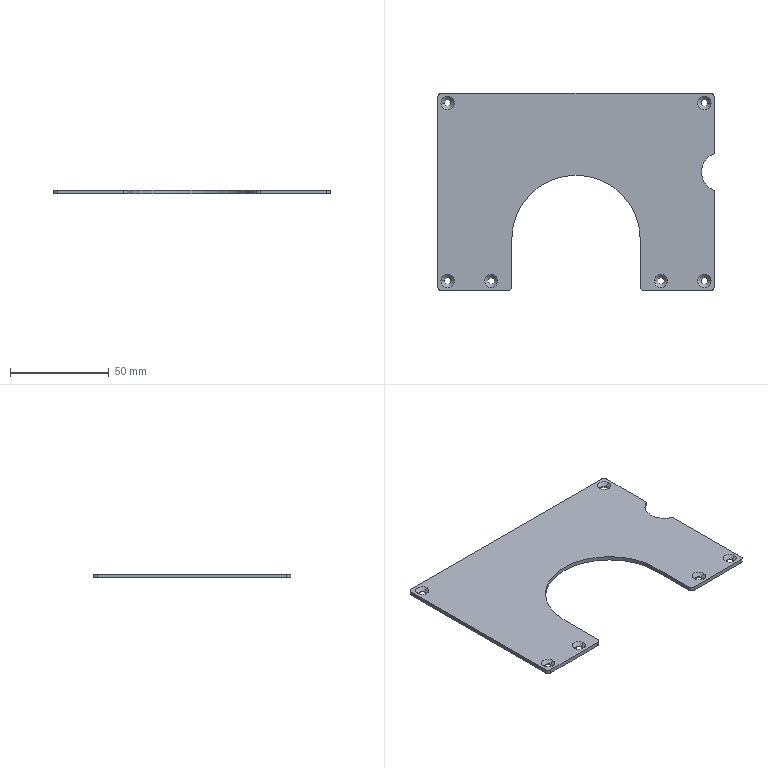Part | STEP file | 11-FG-E03111 | 1 solid | 42 faces | box 140 x 100 x 2 mm | volume 20888 mm3 | cylinder 20 | cone 12 | plane 10 | commonest cylinder face diameters 3.4 x12 4 x6 20 x1 65 x1
STEP:
#1=CARTESIAN_POINT('',(-66.7,45.,0.34));
#2=VERTEX_POINT('',#1);
#3=CARTESIAN_POINT('',(-63.3,45.,0.34));
#4=VERTEX_POINT('',#3);
#5=CARTESIAN_POINT('',(-65.,45.,0.34));
#6=DIRECTION('',(0.,0.,1.));
#7=DIRECTION('',(1.,0.,0.));
#8=AXIS2_PLACEMENT_3D('',#5,#6,#7);
#9=CIRCLE('',#8,1.7);
#10=EDGE_CURVE('',#2,#4,#9,.T.);
#11=ORIENTED_EDGE('',*,*,#10,.F.);
#12=CARTESIAN_POINT('',(-68.36,45.,2.));
#13=VERTEX_POINT('',#12);
#14=CARTESIAN_POINT('',(-68.36,45.,2.));
#15=DIRECTION('',(-0.7071,0.,0.7071));
#16=VECTOR('',#15,1000.);
#17=LINE('',#14,#16);
#18=EDGE_CURVE('',#2,#13,#17,.T.);
#19=ORIENTED_EDGE('',*,*,#18,.T.);
#20=CARTESIAN_POINT('',(-61.64,45.,2.));
#21=VERTEX_POINT('',#20);
#22=CARTESIAN_POINT('',(-65.,45.,2.));
#23=DIRECTION('',(0.,0.,1.));
#24=DIRECTION('',(1.,0.,0.));
#25=AXIS2_PLACEMENT_3D('',#22,#23,#24);
#26=CIRCLE('',#25,3.36);
#27=EDGE_CURVE('',#13,#21,#26,.T.);
#28=ORIENTED_EDGE('',*,*,#27,.T.);
#29=CARTESIAN_POINT('',(-61.64,45.,2.));
#30=DIRECTION('',(0.7071,0.,0.7071));
#31=VECTOR('',#30,1000.);
#32=LINE('',#29,#31);
#33=EDGE_CURVE('',#4,#21,#32,.T.);
#34=ORIENTED_EDGE('',*,*,#33,.F.);
#35=EDGE_LOOP('',(#11,#19,#28,#34));
#36=FACE_OUTER_BOUND('',#35,.T.);
#37=CARTESIAN_POINT('',(-65.,45.,2.));
#38=DIRECTION('',(0.,0.,1.));
#39=DIRECTION('',(1.,0.,0.));
#40=AXIS2_PLACEMENT_3D('',#37,#38,#39);
#41=CONICAL_SURFACE('',#40,3.36,0.7854);
#42=ADVANCED_FACE('',(#36),#41,.F.);
#43=CARTESIAN_POINT('',(-66.7,45.,0.));
#44=VERTEX_POINT('',#43);
#45=CARTESIAN_POINT('',(-63.3,45.,0.));
#46=VERTEX_POINT('',#45);
#47=CARTESIAN_POINT('',(-65.,45.,0.));
#48=DIRECTION('',(0.,0.,1.));
#49=DIRECTION('',(1.,0.,0.));
#50=AXIS2_PLACEMENT_3D('',#47,#48,#49);
#51=CIRCLE('',#50,1.7);
#52=EDGE_CURVE('',#44,#46,#51,.T.);
#53=ORIENTED_EDGE('',*,*,#52,.F.);
#54=CARTESIAN_POINT('',(-66.7,45.,2.));
#55=DIRECTION('',(0.,0.,1.));
#56=VECTOR('',#55,1000.);
#57=LINE('',#54,#56);
#58=EDGE_CURVE('',#44,#2,#57,.T.);
#59=ORIENTED_EDGE('',*,*,#58,.T.);
#60=ORIENTED_EDGE('',*,*,#10,.T.);
#61=CARTESIAN_POINT('',(-63.3,45.,2.));
#62=DIRECTION('',(0.,0.,1.));
#63=VECTOR('',#62,1000.);
#64=LINE('',#61,#63);
#65=EDGE_CURVE('',#46,#4,#64,.T.);
#66=ORIENTED_EDGE('',*,*,#65,.F.);
#67=EDGE_LOOP('',(#53,#59,#60,#66));
#68=FACE_OUTER_BOUND('',#67,.T.);
#69=CARTESIAN_POINT('',(-65.,45.,2.));
#70=DIRECTION('',(0.,0.,1.));
#71=DIRECTION('',(1.,0.,0.));
#72=AXIS2_PLACEMENT_3D('',#69,#70,#71);
#73=CYLINDRICAL_SURFACE('',#72,1.7);
#74=ADVANCED_FACE('',(#68),#73,.F.);
#75=CARTESIAN_POINT('',(63.3,45.,0.34));
#76=VERTEX_POINT('',#75);
#77=CARTESIAN_POINT('',(66.7,45.,0.34));
#78=VERTEX_POINT('',#77);
#79=CARTESIAN_POINT('',(65.,45.,0.34));
#80=DIRECTION('',(0.,0.,1.));
#81=DIRECTION('',(1.,0.,0.));
#82=AXIS2_PLACEMENT_3D('',#79,#80,#81);
#83=CIRCLE('',#82,1.7);
#84=EDGE_CURVE('',#76,#78,#83,.T.);
#85=ORIENTED_EDGE('',*,*,#84,.F.);
#86=CARTESIAN_POINT('',(61.64,45.,2.));
#87=VERTEX_POINT('',#86);
#88=CARTESIAN_POINT('',(61.64,45.,2.));
#89=DIRECTION('',(-0.7071,0.,0.7071));
#90=VECTOR('',#89,1000.);
#91=LINE('',#88,#90);
#92=EDGE_CURVE('',#76,#87,#91,.T.);
#93=ORIENTED_EDGE('',*,*,#92,.T.);
#94=CARTESIAN_POINT('',(68.36,45.,2.));
#95=VERTEX_POINT('',#94);
#96=CARTESIAN_POINT('',(65.,45.,2.));
#97=DIRECTION('',(0.,0.,1.));
#98=DIRECTION('',(1.,0.,0.));
#99=AXIS2_PLACEMENT_3D('',#96,#97,#98);
#100=CIRCLE('',#99,3.36);
#101=EDGE_CURVE('',#87,#95,#100,.T.);
#102=ORIENTED_EDGE('',*,*,#101,.T.);
#103=CARTESIAN_POINT('',(68.36,45.,2.));
#104=DIRECTION('',(0.7071,0.,0.7071));
#105=VECTOR('',#104,1000.);
#106=LINE('',#103,#105);
#107=EDGE_CURVE('',#78,#95,#106,.T.);
#108=ORIENTED_EDGE('',*,*,#107,.F.);
#109=EDGE_LOOP('',(#85,#93,#102,#108));
#110=FACE_OUTER_BOUND('',#109,.T.);
#111=CARTESIAN_POINT('',(65.,45.,2.));
#112=DIRECTION('',(0.,0.,1.));
#113=DIRECTION('',(1.,0.,0.));
#114=AXIS2_PLACEMENT_3D('',#111,#112,#113);
#115=CONICAL_SURFACE('',#114,3.36,0.7854);
#116=ADVANCED_FACE('',(#110),#115,.F.);
#117=CARTESIAN_POINT('',(63.3,45.,0.));
#118=VERTEX_POINT('',#117);
#119=CARTESIAN_POINT('',(66.7,45.,0.));
#120=VERTEX_POINT('',#119);
#121=CARTESIAN_POINT('',(65.,45.,0.));
#122=DIRECTION('',(0.,0.,1.));
#123=DIRECTION('',(1.,0.,0.));
#124=AXIS2_PLACEMENT_3D('',#121,#122,#123);
#125=CIRCLE('',#124,1.7);
#126=EDGE_CURVE('',#118,#120,#125,.T.);
#127=ORIENTED_EDGE('',*,*,#126,.F.);
#128=CARTESIAN_POINT('',(63.3,45.,2.));
#129=DIRECTION('',(0.,0.,1.));
#130=VECTOR('',#129,1000.);
#131=LINE('',#128,#130);
#132=EDGE_CURVE('',#118,#76,#131,.T.);
#133=ORIENTED_EDGE('',*,*,#132,.T.);
#134=ORIENTED_EDGE('',*,*,#84,.T.);
#135=CARTESIAN_POINT('',(66.7,45.,2.));
#136=DIRECTION('',(0.,0.,1.));
#137=VECTOR('',#136,1000.);
#138=LINE('',#135,#137);
#139=EDGE_CURVE('',#120,#78,#138,.T.);
#140=ORIENTED_EDGE('',*,*,#139,.F.);
#141=EDGE_LOOP('',(#127,#133,#134,#140));
#142=FACE_OUTER_BOUND('',#141,.T.);
#143=CARTESIAN_POINT('',(65.,45.,2.));
#144=DIRECTION('',(0.,0.,1.));
#145=DIRECTION('',(1.,0.,0.));
#146=AXIS2_PLACEMENT_3D('',#143,#144,#145);
#147=CYLINDRICAL_SURFACE('',#146,1.7);
#148=ADVANCED_FACE('',(#142),#147,.F.);
#149=CARTESIAN_POINT('',(-66.7,-45.,0.34));
#150=VERTEX_POINT('',#149);
#151=CARTESIAN_POINT('',(-63.3,-45.,0.34));
#152=VERTEX_POINT('',#151);
#153=CARTESIAN_POINT('',(-65.,-45.,0.34));
#154=DIRECTION('',(0.,0.,1.));
#155=DIRECTION('',(1.,0.,0.));
#156=AXIS2_PLACEMENT_3D('',#153,#154,#155);
#157=CIRCLE('',#156,1.7);
#158=EDGE_CURVE('',#150,#152,#157,.T.);
#159=ORIENTED_EDGE('',*,*,#158,.F.);
#160=CARTESIAN_POINT('',(-68.36,-45.,2.));
#161=VERTEX_POINT('',#160);
#162=CARTESIAN_POINT('',(-68.36,-45.,2.));
#163=DIRECTION('',(-0.7071,0.,0.7071));
#164=VECTOR('',#163,1000.);
#165=LINE('',#162,#164);
#166=EDGE_CURVE('',#150,#161,#165,.T.);
#167=ORIENTED_EDGE('',*,*,#166,.T.);
#168=CARTESIAN_POINT('',(-61.64,-45.,2.));
#169=VERTEX_POINT('',#168);
#170=CARTESIAN_POINT('',(-65.,-45.,2.));
#171=DIRECTION('',(0.,0.,1.));
#172=DIRECTION('',(1.,0.,0.));
#173=AXIS2_PLACEMENT_3D('',#170,#171,#172);
#174=CIRCLE('',#173,3.36);
#175=EDGE_CURVE('',#161,#169,#174,.T.);
#176=ORIENTED_EDGE('',*,*,#175,.T.);
#177=CARTESIAN_POINT('',(-61.64,-45.,2.));
#178=DIRECTION('',(0.7071,0.,0.7071));
#179=VECTOR('',#178,1000.);
#180=LINE('',#177,#179);
#181=EDGE_CURVE('',#152,#169,#180,.T.);
#182=ORIENTED_EDGE('',*,*,#181,.F.);
#183=EDGE_LOOP('',(#159,#167,#176,#182));
#184=FACE_OUTER_BOUND('',#183,.T.);
#185=CARTESIAN_POINT('',(-65.,-45.,2.));
#186=DIRECTION('',(0.,0.,1.));
#187=DIRECTION('',(1.,0.,0.));
#188=AXIS2_PLACEMENT_3D('',#185,#186,#187);
#189=CONICAL_SURFACE('',#188,3.36,0.7854);
#190=ADVANCED_FACE('',(#184),#189,.F.);
#191=CARTESIAN_POINT('',(-66.7,-45.,0.));
#192=VERTEX_POINT('',#191);
#193=CARTESIAN_POINT('',(-63.3,-45.,0.));
#194=VERTEX_POINT('',#193);
#195=CARTESIAN_POINT('',(-65.,-45.,0.));
#196=DIRECTION('',(0.,0.,1.));
#197=DIRECTION('',(1.,0.,0.));
#198=AXIS2_PLACEMENT_3D('',#195,#196,#197);
#199=CIRCLE('',#198,1.7);
#200=EDGE_CURVE('',#192,#194,#199,.T.);
#201=ORIENTED_EDGE('',*,*,#200,.F.);
#202=CARTESIAN_POINT('',(-66.7,-45.,2.));
#203=DIRECTION('',(0.,0.,1.));
#204=VECTOR('',#203,1000.);
#205=LINE('',#202,#204);
#206=EDGE_CURVE('',#192,#150,#205,.T.);
#207=ORIENTED_EDGE('',*,*,#206,.T.);
#208=ORIENTED_EDGE('',*,*,#158,.T.);
#209=CARTESIAN_POINT('',(-63.3,-45.,2.));
#210=DIRECTION('',(0.,0.,1.));
#211=VECTOR('',#210,1000.);
#212=LINE('',#209,#211);
#213=EDGE_CURVE('',#194,#152,#212,.T.);
#214=ORIENTED_EDGE('',*,*,#213,.F.);
#215=EDGE_LOOP('',(#201,#207,#208,#214));
#216=FACE_OUTER_BOUND('',#215,.T.);
#217=CARTESIAN_POINT('',(-65.,-45.,2.));
#218=DIRECTION('',(0.,0.,1.));
#219=DIRECTION('',(1.,0.,0.));
#220=AXIS2_PLACEMENT_3D('',#217,#218,#219);
#221=CYLINDRICAL_SURFACE('',#220,1.7);
#222=ADVANCED_FACE('',(#216),#221,.F.);
#223=CARTESIAN_POINT('',(-44.7,-45.,0.34));
#224=VERTEX_POINT('',#223);
#225=CARTESIAN_POINT('',(-41.3,-45.,0.34));
#226=VERTEX_POINT('',#225);
#227=CARTESIAN_POINT('',(-43.,-45.,0.34));
#228=DIRECTION('',(0.,0.,1.));
#229=DIRECTION('',(1.,0.,0.));
#230=AXIS2_PLACEMENT_3D('',#227,#228,#229);
#231=CIRCLE('',#230,1.7);
#232=EDGE_CURVE('',#224,#226,#231,.T.);
#233=ORIENTED_EDGE('',*,*,#232,.F.);
#234=CARTESIAN_POINT('',(-46.36,-45.,2.));
#235=VERTEX_POINT('',#234);
#236=CARTESIAN_POINT('',(-46.36,-45.,2.));
#237=DIRECTION('',(-0.7071,0.,0.7071));
#238=VECTOR('',#237,1000.);
#239=LINE('',#236,#238);
#240=EDGE_CURVE('',#224,#235,#239,.T.);
#241=ORIENTED_EDGE('',*,*,#240,.T.);
#242=CARTESIAN_POINT('',(-39.64,-45.,2.));
#243=VERTEX_POINT('',#242);
#244=CARTESIAN_POINT('',(-43.,-45.,2.));
#245=DIRECTION('',(0.,0.,1.));
#246=DIRECTION('',(1.,0.,0.));
#247=AXIS2_PLACEMENT_3D('',#244,#245,#246);
#248=CIRCLE('',#247,3.36);
#249=EDGE_CURVE('',#235,#243,#248,.T.);
#250=ORIENTED_EDGE('',*,*,#249,.T.);
#251=CARTESIAN_POINT('',(-39.64,-45.,2.));
#252=DIRECTION('',(0.7071,0.,0.7071));
#253=VECTOR('',#252,1000.);
#254=LINE('',#251,#253);
#255=EDGE_CURVE('',#226,#243,#254,.T.);
#256=ORIENTED_EDGE('',*,*,#255,.F.);
#257=EDGE_LOOP('',(#233,#241,#250,#256));
#258=FACE_OUTER_BOUND('',#257,.T.);
#259=CARTESIAN_POINT('',(-43.,-45.,2.));
#260=DIRECTION('',(0.,0.,1.));
#261=DIRECTION('',(1.,0.,0.));
#262=AXIS2_PLACEMENT_3D('',#259,#260,#261);
#263=CONICAL_SURFACE('',#262,3.36,0.7854);
#264=ADVANCED_FACE('',(#258),#263,.F.);
#265=CARTESIAN_POINT('',(-44.7,-45.,0.));
#266=VERTEX_POINT('',#265);
#267=CARTESIAN_POINT('',(-41.3,-45.,0.));
#268=VERTEX_POINT('',#267);
#269=CARTESIAN_POINT('',(-43.,-45.,0.));
#270=DIRECTION('',(0.,0.,1.));
#271=DIRECTION('',(1.,0.,0.));
#272=AXIS2_PLACEMENT_3D('',#269,#270,#271);
#273=CIRCLE('',#272,1.7);
#274=EDGE_CURVE('',#266,#268,#273,.T.);
#275=ORIENTED_EDGE('',*,*,#274,.F.);
#276=CARTESIAN_POINT('',(-44.7,-45.,2.));
#277=DIRECTION('',(0.,0.,1.));
#278=VECTOR('',#277,1000.);
#279=LINE('',#276,#278);
#280=EDGE_CURVE('',#266,#224,#279,.T.);
#281=ORIENTED_EDGE('',*,*,#280,.T.);
#282=ORIENTED_EDGE('',*,*,#232,.T.);
#283=CARTESIAN_POINT('',(-41.3,-45.,2.));
#284=DIRECTION('',(0.,0.,1.));
#285=VECTOR('',#284,1000.);
#286=LINE('',#283,#285);
#287=EDGE_CURVE('',#268,#226,#286,.T.);
#288=ORIENTED_EDGE('',*,*,#287,.F.);
#289=EDGE_LOOP('',(#275,#281,#282,#288));
#290=FACE_OUTER_BOUND('',#289,.T.);
#291=CARTESIAN_POINT('',(-43.,-45.,2.));
#292=DIRECTION('',(0.,0.,1.));
#293=DIRECTION('',(1.,0.,0.));
#294=AXIS2_PLACEMENT_3D('',#291,#292,#293);
#295=CYLINDRICAL_SURFACE('',#294,1.7);
#296=ADVANCED_FACE('',(#290),#295,.F.);
#297=CARTESIAN_POINT('',(41.3,-45.,0.34));
#298=VERTEX_POINT('',#297);
#299=CARTESIAN_POINT('',(44.7,-45.,0.34));
#300=VERTEX_POINT('',#299);
#301=CARTESIAN_POINT('',(43.,-45.,0.34));
#302=DIRECTION('',(0.,0.,1.));
#303=DIRECTION('',(1.,0.,0.));
#304=AXIS2_PLACEMENT_3D('',#301,#302,#303);
#305=CIRCLE('',#304,1.7);
#306=EDGE_CURVE('',#298,#300,#305,.T.);
#307=ORIENTED_EDGE('',*,*,#306,.F.);
#308=CARTESIAN_POINT('',(39.64,-45.,2.));
#309=VERTEX_POINT('',#308);
#310=CARTESIAN_POINT('',(39.64,-45.,2.));
#311=DIRECTION('',(-0.7071,0.,0.7071));
#312=VECTOR('',#311,1000.);
#313=LINE('',#310,#312);
#314=EDGE_CURVE('',#298,#309,#313,.T.);
#315=ORIENTED_EDGE('',*,*,#314,.T.);
#316=CARTESIAN_POINT('',(46.36,-45.,2.));
#317=VERTEX_POINT('',#316);
#318=CARTESIAN_POINT('',(43.,-45.,2.));
#319=DIRECTION('',(0.,0.,1.));
#320=DIRECTION('',(1.,0.,0.));
#321=AXIS2_PLACEMENT_3D('',#318,#319,#320);
#322=CIRCLE('',#321,3.36);
#323=EDGE_CURVE('',#309,#317,#322,.T.);
#324=ORIENTED_EDGE('',*,*,#323,.T.);
#325=CARTESIAN_POINT('',(46.36,-45.,2.));
#326=DIRECTION('',(0.7071,0.,0.7071));
#327=VECTOR('',#326,1000.);
#328=LINE('',#325,#327);
#329=EDGE_CURVE('',#300,#317,#328,.T.);
#330=ORIENTED_EDGE('',*,*,#329,.F.);
#331=EDGE_LOOP('',(#307,#315,#324,#330));
#332=FACE_OUTER_BOUND('',#331,.T.);
#333=CARTESIAN_POINT('',(43.,-45.,2.));
#334=DIRECTION('',(0.,0.,1.));
#335=DIRECTION('',(1.,0.,0.));
#336=AXIS2_PLACEMENT_3D('',#333,#334,#335);
#337=CONICAL_SURFACE('',#336,3.36,0.7854);
#338=ADVANCED_FACE('',(#332),#337,.F.);
#339=CARTESIAN_POINT('',(41.3,-45.,0.));
#340=VERTEX_POINT('',#339);
#341=CARTESIAN_POINT('',(44.7,-45.,0.));
#342=VERTEX_POINT('',#341);
#343=CARTESIAN_POINT('',(43.,-45.,0.));
#344=DIRECTION('',(0.,0.,1.));
#345=DIRECTION('',(1.,0.,0.));
#346=AXIS2_PLACEMENT_3D('',#343,#344,#345);
#347=CIRCLE('',#346,1.7);
#348=EDGE_CURVE('',#340,#342,#347,.T.);
#349=ORIENTED_EDGE('',*,*,#348,.F.);
#350=CARTESIAN_POINT('',(41.3,-45.,2.));
#351=DIRECTION('',(0.,0.,1.));
#352=VECTOR('',#351,1000.);
#353=LINE('',#350,#352);
#354=EDGE_CURVE('',#340,#298,#353,.T.);
#355=ORIENTED_EDGE('',*,*,#354,.T.);
#356=ORIENTED_EDGE('',*,*,#306,.T.);
#357=CARTESIAN_POINT('',(44.7,-45.,2.));
#358=DIRECTION('',(0.,0.,1.));
#359=VECTOR('',#358,1000.);
#360=LINE('',#357,#359);
#361=EDGE_CURVE('',#342,#300,#360,.T.);
#362=ORIENTED_EDGE('',*,*,#361,.F.);
#363=EDGE_LOOP('',(#349,#355,#356,#362));
#364=FACE_OUTER_BOUND('',#363,.T.);
#365=CARTESIAN_POINT('',(43.,-45.,2.));
#366=DIRECTION('',(0.,0.,1.));
#367=DIRECTION('',(1.,0.,0.));
#368=AXIS2_PLACEMENT_3D('',#365,#366,#367);
#369=CYLINDRICAL_SURFACE('',#368,1.7);
#370=ADVANCED_FACE('',(#364),#369,.F.);
#371=CARTESIAN_POINT('',(63.3,-45.,0.34));
#372=VERTEX_POINT('',#371);
#373=CARTESIAN_POINT('',(66.7,-45.,0.34));
#374=VERTEX_POINT('',#373);
#375=CARTESIAN_POINT('',(65.,-45.,0.34));
#376=DIRECTION('',(0.,0.,1.));
#377=DIRECTION('',(1.,0.,0.));
#378=AXIS2_PLACEMENT_3D('',#375,#376,#377);
#379=CIRCLE('',#378,1.7);
#380=EDGE_CURVE('',#372,#374,#379,.T.);
#381=ORIENTED_EDGE('',*,*,#380,.F.);
#382=CARTESIAN_POINT('',(61.64,-45.,2.));
#383=VERTEX_POINT('',#382);
#384=CARTESIAN_POINT('',(61.64,-45.,2.));
#385=DIRECTION('',(-0.7071,0.,0.7071));
#386=VECTOR('',#385,1000.);
#387=LINE('',#384,#386);
#388=EDGE_CURVE('',#372,#383,#387,.T.);
#389=ORIENTED_EDGE('',*,*,#388,.T.);
#390=CARTESIAN_POINT('',(68.36,-45.,2.));
#391=VERTEX_POINT('',#390);
#392=CARTESIAN_POINT('',(65.,-45.,2.));
#393=DIRECTION('',(0.,0.,1.));
#394=DIRECTION('',(1.,0.,0.));
#395=AXIS2_PLACEMENT_3D('',#392,#393,#394);
#396=CIRCLE('',#395,3.36);
#397=EDGE_CURVE('',#383,#391,#396,.T.);
#398=ORIENTED_EDGE('',*,*,#397,.T.);
#399=CARTESIAN_POINT('',(68.36,-45.,2.));
#400=DIRECTION('',(0.7071,0.,0.7071));
#401=VECTOR('',#400,1000.);
#402=LINE('',#399,#401);
#403=EDGE_CURVE('',#374,#391,#402,.T.);
#404=ORIENTED_EDGE('',*,*,#403,.F.);
#405=EDGE_LOOP('',(#381,#389,#398,#404));
#406=FACE_OUTER_BOUND('',#405,.T.);
#407=CARTESIAN_POINT('',(65.,-45.,2.));
#408=DIRECTION('',(0.,0.,1.));
#409=DIRECTION('',(1.,0.,0.));
#410=AXIS2_PLACEMENT_3D('',#407,#408,#409);
#411=CONICAL_SURFACE('',#410,3.36,0.7854);
#412=ADVANCED_FACE('',(#406),#411,.F.);
#413=CARTESIAN_POINT('',(63.3,-45.,0.));
#414=VERTEX_POINT('',#413);
#415=CARTESIAN_POINT('',(66.7,-45.,0.));
#416=VERTEX_POINT('',#415);
#417=CARTESIAN_POINT('',(65.,-45.,0.));
#418=DIRECTION('',(0.,0.,1.));
#419=DIRECTION('',(1.,0.,0.));
#420=AXIS2_PLACEMENT_3D('',#417,#418,#419);
#421=CIRCLE('',#420,1.7);
#422=EDGE_CURVE('',#414,#416,#421,.T.);
#423=ORIENTED_EDGE('',*,*,#422,.F.);
#424=CARTESIAN_POINT('',(63.3,-45.,2.));
#425=DIRECTION('',(0.,0.,1.));
#426=VECTOR('',#425,1000.);
#427=LINE('',#424,#426);
#428=EDGE_CURVE('',#414,#372,#427,.T.);
#429=ORIENTED_EDGE('',*,*,#428,.T.);
#430=ORIENTED_EDGE('',*,*,#380,.T.);
#431=CARTESIAN_POINT('',(66.7,-45.,2.));
#432=DIRECTION('',(0.,0.,1.));
#433=VECTOR('',#432,1000.);
#434=LINE('',#431,#433);
#435=EDGE_CURVE('',#416,#374,#434,.T.);
#436=ORIENTED_EDGE('',*,*,#435,.F.);
#437=EDGE_LOOP('',(#423,#429,#430,#436));
#438=FACE_OUTER_BOUND('',#437,.T.);
#439=CARTESIAN_POINT('',(65.,-45.,2.));
#440=DIRECTION('',(0.,0.,1.));
#441=DIRECTION('',(1.,0.,0.));
#442=AXIS2_PLACEMENT_3D('',#439,#440,#441);
#443=CYLINDRICAL_SURFACE('',#442,1.7);
#444=ADVANCED_FACE('',(#438),#443,.F.);
#445=CARTESIAN_POINT('',(70.,-48.,0.));
#446=VERTEX_POINT('',#445);
#447=CARTESIAN_POINT('',(70.,0.7075,0.));
#448=VERTEX_POINT('',#447);
#449=CARTESIAN_POINT('',(70.,50.,0.));
#450=DIRECTION('',(0.,1.,0.));
#451=VECTOR('',#450,1000.);
#452=LINE('',#449,#451);
#453=EDGE_CURVE('',#446,#448,#452,.T.);
#454=ORIENTED_EDGE('',*,*,#453,.T.);
#455=CARTESIAN_POINT('',(70.,0.7075,2.));
#456=VERTEX_POINT('',#455);
#457=CARTESIAN_POINT('',(70.,0.7075,0.));
#458=DIRECTION('',(0.,0.,1.));
#459=VECTOR('',#458,1000.);
#460=LINE('',#457,#459);
#461=EDGE_CURVE('',#448,#456,#460,.T.);
#462=ORIENTED_EDGE('',*,*,#461,.T.);
#463=CARTESIAN_POINT('',(70.,-48.,2.));
#464=VERTEX_POINT('',#463);
#465=CARTESIAN_POINT('',(70.,50.,2.));
#466=DIRECTION('',(0.,1.,0.));
#467=VECTOR('',#466,1000.);
#468=LINE('',#465,#467);
#469=EDGE_CURVE('',#464,#456,#468,.T.);
#470=ORIENTED_EDGE('',*,*,#469,.F.);
#471=CARTESIAN_POINT('',(70.,-48.,2.));
#472=DIRECTION('',(0.,0.,-1.));
#473=VECTOR('',#472,1000.);
#474=LINE('',#471,#473);
#475=EDGE_CURVE('',#464,#446,#474,.T.);
#476=ORIENTED_EDGE('',*,*,#475,.T.);
#477=EDGE_LOOP('',(#454,#462,#470,#476));
#478=FACE_OUTER_BOUND('',#477,.T.);
#479=CARTESIAN_POINT('',(70.,50.,2.));
#480=DIRECTION('',(-1.,0.,0.));
#481=DIRECTION('',(0.,0.,1.));
#482=AXIS2_PLACEMENT_3D('',#479,#480,#481);
#483=PLANE('',#482);
#484=ADVANCED_FACE('',(#478),#483,.F.);
#485=CARTESIAN_POINT('',(34.5,-50.,2.));
#486=VERTEX_POINT('',#485);
#487=CARTESIAN_POINT('',(68.,-50.,2.));
#488=VERTEX_POINT('',#487);
#489=CARTESIAN_POINT('',(-70.,-50.,2.));
#490=DIRECTION('',(1.,0.,0.));
#491=VECTOR('',#490,1000.);
#492=LINE('',#489,#491);
#493=EDGE_CURVE('',#486,#488,#492,.T.);
#494=ORIENTED_EDGE('',*,*,#493,.F.);
#495=CARTESIAN_POINT('',(34.5,-50.,0.));
#496=VERTEX_POINT('',#495);
#497=CARTESIAN_POINT('',(34.5,-50.,2.));
#498=DIRECTION('',(0.,0.,-1.));
#499=VECTOR('',#498,1000.);
#500=LINE('',#497,#499);
#501=EDGE_CURVE('',#486,#496,#500,.T.);
#502=ORIENTED_EDGE('',*,*,#501,.T.);
#503=CARTESIAN_POINT('',(68.,-50.,0.));
#504=VERTEX_POINT('',#503);
#505=CARTESIAN_POINT('',(-70.,-50.,0.));
#506=DIRECTION('',(1.,0.,0.));
#507=VECTOR('',#506,1000.);
#508=LINE('',#505,#507);
#509=EDGE_CURVE('',#496,#504,#508,.T.);
#510=ORIENTED_EDGE('',*,*,#509,.T.);
#511=CARTESIAN_POINT('',(68.,-50.,2.));
#512=DIRECTION('',(0.,0.,1.));
#513=VECTOR('',#512,1000.);
#514=LINE('',#511,#513);
#515=EDGE_CURVE('',#504,#488,#514,.T.);
#516=ORIENTED_EDGE('',*,*,#515,.T.);
#517=EDGE_LOOP('',(#494,#502,#510,#516));
#518=FACE_OUTER_BOUND('',#517,.T.);
#519=CARTESIAN_POINT('',(-70.,-50.,2.));
#520=DIRECTION('',(0.,1.,0.));
#521=DIRECTION('',(0.,0.,1.));
#522=AXIS2_PLACEMENT_3D('',#519,#520,#521);
#523=PLANE('',#522);
#524=ADVANCED_FACE('',(#518),#523,.F.);
#525=CARTESIAN_POINT('',(70.,19.442,2.));
#526=VERTEX_POINT('',#525);
#527=CARTESIAN_POINT('',(70.,48.,2.));
#528=VERTEX_POINT('',#527);
#529=CARTESIAN_POINT('',(70.,50.,2.));
#530=DIRECTION('',(0.,1.,0.));
#531=VECTOR('',#530,1000.);
#532=LINE('',#529,#531);
#533=EDGE_CURVE('',#526,#528,#532,.T.);
#534=ORIENTED_EDGE('',*,*,#533,.F.);
#535=CARTESIAN_POINT('',(70.,19.442,0.));
#536=VERTEX_POINT('',#535);
#537=CARTESIAN_POINT('',(70.,19.442,0.));
#538=DIRECTION('',(0.,0.,-1.));
#539=VECTOR('',#538,1000.);
#540=LINE('',#537,#539);
#541=EDGE_CURVE('',#526,#536,#540,.T.);
#542=ORIENTED_EDGE('',*,*,#541,.T.);
#543=CARTESIAN_POINT('',(70.,48.,0.));
#544=VERTEX_POINT('',#543);
#545=CARTESIAN_POINT('',(70.,50.,0.));
#546=DIRECTION('',(0.,1.,0.));
#547=VECTOR('',#546,1000.);
#548=LINE('',#545,#547);
#549=EDGE_CURVE('',#536,#544,#548,.T.);
#550=ORIENTED_EDGE('',*,*,#549,.T.);
#551=CARTESIAN_POINT('',(70.,48.,2.));
#552=DIRECTION('',(0.,0.,1.));
#553=VECTOR('',#552,1000.);
#554=LINE('',#551,#553);
#555=EDGE_CURVE('',#544,#528,#554,.T.);
#556=ORIENTED_EDGE('',*,*,#555,.T.);
#557=EDGE_LOOP('',(#534,#542,#550,#556));
#558=FACE_OUTER_BOUND('',#557,.T.);
#559=CARTESIAN_POINT('',(70.,50.,2.));
#560=DIRECTION('',(-1.,0.,0.));
#561=DIRECTION('',(0.,0.,1.));
#562=AXIS2_PLACEMENT_3D('',#559,#560,#561);
#563=PLANE('',#562);
#564=ADVANCED_FACE('',(#558),#563,.F.);
#565=CARTESIAN_POINT('',(68.,50.,2.));
#566=VERTEX_POINT('',#565);
#567=CARTESIAN_POINT('',(-68.,50.,2.));
#568=VERTEX_POINT('',#567);
#569=CARTESIAN_POINT('',(-70.,50.,2.));
#570=DIRECTION('',(-1.,0.,0.));
#571=VECTOR('',#570,1000.);
#572=LINE('',#569,#571);
#573=EDGE_CURVE('',#566,#568,#572,.T.);
#574=ORIENTED_EDGE('',*,*,#573,.F.);
#575=CARTESIAN_POINT('',(68.,50.,0.));
#576=VERTEX_POINT('',#575);
#577=CARTESIAN_POINT('',(68.,50.,2.));
#578=DIRECTION('',(0.,0.,-1.));
#579=VECTOR('',#578,1000.);
#580=LINE('',#577,#579);
#581=EDGE_CURVE('',#566,#576,#580,.T.);
#582=ORIENTED_EDGE('',*,*,#581,.T.);
#583=CARTESIAN_POINT('',(-68.,50.,0.));
#584=VERTEX_POINT('',#583);
#585=CARTESIAN_POINT('',(-70.,50.,0.));
#586=DIRECTION('',(-1.,0.,0.));
#587=VECTOR('',#586,1000.);
#588=LINE('',#585,#587);
#589=EDGE_CURVE('',#576,#584,#588,.T.);
#590=ORIENTED_EDGE('',*,*,#589,.T.);
#591=CARTESIAN_POINT('',(-68.,50.,2.));
#592=DIRECTION('',(0.,0.,1.));
#593=VECTOR('',#592,1000.);
#594=LINE('',#591,#593);
#595=EDGE_CURVE('',#584,#568,#594,.T.);
#596=ORIENTED_EDGE('',*,*,#595,.T.);
#597=EDGE_LOOP('',(#574,#582,#590,#596));
#598=FACE_OUTER_BOUND('',#597,.T.);
#599=CARTESIAN_POINT('',(-70.,50.,2.));
#600=DIRECTION('',(0.,-1.,0.));
#601=DIRECTION('',(0.,0.,-1.));
#602=AXIS2_PLACEMENT_3D('',#599,#600,#601);
#603=PLANE('',#602);
#604=ADVANCED_FACE('',(#598),#603,.F.);
#605=CARTESIAN_POINT('',(-70.,48.,0.));
#606=VERTEX_POINT('',#605);
#607=CARTESIAN_POINT('',(-70.,-48.,0.));
#608=VERTEX_POINT('',#607);
#609=CARTESIAN_POINT('',(-70.,50.,0.));
#610=DIRECTION('',(0.,-1.,0.));
#611=VECTOR('',#610,1000.);
#612=LINE('',#609,#611);
#613=EDGE_CURVE('',#606,#608,#612,.T.);
#614=ORIENTED_EDGE('',*,*,#613,.T.);
#615=CARTESIAN_POINT('',(-70.,-48.,2.));
#616=VERTEX_POINT('',#615);
#617=CARTESIAN_POINT('',(-70.,-48.,2.));
#618=DIRECTION('',(0.,0.,1.));
#619=VECTOR('',#618,1000.);
#620=LINE('',#617,#619);
#621=EDGE_CURVE('',#608,#616,#620,.T.);
#622=ORIENTED_EDGE('',*,*,#621,.T.);
#623=CARTESIAN_POINT('',(-70.,48.,2.));
#624=VERTEX_POINT('',#623);
#625=CARTESIAN_POINT('',(-70.,50.,2.));
#626=DIRECTION('',(0.,-1.,0.));
#627=VECTOR('',#626,1000.);
#628=LINE('',#625,#627);
#629=EDGE_CURVE('',#624,#616,#628,.T.);
#630=ORIENTED_EDGE('',*,*,#629,.F.);
#631=CARTESIAN_POINT('',(-70.,48.,2.));
#632=DIRECTION('',(0.,0.,-1.));
#633=VECTOR('',#632,1000.);
#634=LINE('',#631,#633);
#635=EDGE_CURVE('',#624,#606,#634,.T.);
#636=ORIENTED_EDGE('',*,*,#635,.T.);
#637=EDGE_LOOP('',(#614,#622,#630,#636));
#638=FACE_OUTER_BOUND('',#637,.T.);
#639=CARTESIAN_POINT('',(-70.,50.,2.));
#640=DIRECTION('',(1.,0.,0.));
#641=DIRECTION('',(0.,0.,-1.));
#642=AXIS2_PLACEMENT_3D('',#639,#640,#641);
#643=PLANE('',#642);
#644=ADVANCED_FACE('',(#638),#643,.F.);
#645=CARTESIAN_POINT('',(-68.,-50.,2.));
#646=VERTEX_POINT('',#645);
#647=CARTESIAN_POINT('',(-34.5,-50.,2.));
#648=VERTEX_POINT('',#647);
#649=CARTESIAN_POINT('',(-70.,-50.,2.));
#650=DIRECTION('',(1.,0.,0.));
#651=VECTOR('',#650,1000.);
#652=LINE('',#649,#651);
#653=EDGE_CURVE('',#646,#648,#652,.T.);
#654=ORIENTED_EDGE('',*,*,#653,.F.);
#655=CARTESIAN_POINT('',(-68.,-50.,0.));
#656=VERTEX_POINT('',#655);
#657=CARTESIAN_POINT('',(-68.,-50.,2.));
#658=DIRECTION('',(0.,0.,-1.));
#659=VECTOR('',#658,1000.);
#660=LINE('',#657,#659);
#661=EDGE_CURVE('',#646,#656,#660,.T.);
#662=ORIENTED_EDGE('',*,*,#661,.T.);
#663=CARTESIAN_POINT('',(-34.5,-50.,0.));
#664=VERTEX_POINT('',#663);
#665=CARTESIAN_POINT('',(-70.,-50.,0.));
#666=DIRECTION('',(1.,0.,0.));
#667=VECTOR('',#666,1000.);
#668=LINE('',#665,#667);
#669=EDGE_CURVE('',#656,#664,#668,.T.);
#670=ORIENTED_EDGE('',*,*,#669,.T.);
#671=CARTESIAN_POINT('',(-34.5,-50.,2.));
#672=DIRECTION('',(0.,0.,1.));
#673=VECTOR('',#672,1000.);
#674=LINE('',#671,#673);
#675=EDGE_CURVE('',#664,#648,#674,.T.);
#676=ORIENTED_EDGE('',*,*,#675,.T.);
#677=EDGE_LOOP('',(#654,#662,#670,#676));
#678=FACE_OUTER_BOUND('',#677,.T.);
#679=CARTESIAN_POINT('',(-70.,-50.,2.));
#680=DIRECTION('',(0.,1.,0.));
#681=DIRECTION('',(0.,0.,1.));
#682=AXIS2_PLACEMENT_3D('',#679,#680,#681);
#683=PLANE('',#682);
#684=ADVANCED_FACE('',(#678),#683,.F.);
#685=CARTESIAN_POINT('',(73.5,10.075,2.));
#686=DIRECTION('',(0.,0.,1.));
#687=DIRECTION('',(1.,0.,0.));
#688=AXIS2_PLACEMENT_3D('',#685,#686,#687);
#689=CIRCLE('',#688,10.);
#690=EDGE_CURVE('',#526,#456,#689,.T.);
#691=ORIENTED_EDGE('',*,*,#690,.F.);
#692=ORIENTED_EDGE('',*,*,#533,.T.);
#693=CARTESIAN_POINT('',(68.,48.,2.));
#694=DIRECTION('',(0.,0.,1.));
#695=DIRECTION('',(1.,0.,0.));
#696=AXIS2_PLACEMENT_3D('',#693,#694,#695);
#697=CIRCLE('',#696,2.);
#698=EDGE_CURVE('',#528,#566,#697,.T.);
#699=ORIENTED_EDGE('',*,*,#698,.T.);
#700=ORIENTED_EDGE('',*,*,#573,.T.);
#701=CARTESIAN_POINT('',(-68.,48.,2.));
#702=DIRECTION('',(0.,0.,1.));
#703=DIRECTION('',(1.,0.,0.));
#704=AXIS2_PLACEMENT_3D('',#701,#702,#703);
#705=CIRCLE('',#704,2.);
#706=EDGE_CURVE('',#568,#624,#705,.T.);
#707=ORIENTED_EDGE('',*,*,#706,.T.);
#708=ORIENTED_EDGE('',*,*,#629,.T.);
#709=CARTESIAN_POINT('',(-68.,-48.,2.));
#710=DIRECTION('',(0.,0.,1.));
#711=DIRECTION('',(1.,0.,0.));
#712=AXIS2_PLACEMENT_3D('',#709,#710,#711);
#713=CIRCLE('',#712,2.);
#714=EDGE_CURVE('',#616,#646,#713,.T.);
#715=ORIENTED_EDGE('',*,*,#714,.T.);
#716=ORIENTED_EDGE('',*,*,#653,.T.);
#717=CARTESIAN_POINT('',(-32.5,-48.,2.));
#718=VERTEX_POINT('',#717);
#719=CARTESIAN_POINT('',(-34.5,-48.,2.));
#720=DIRECTION('',(0.,0.,1.));
#721=DIRECTION('',(1.,0.,0.));
#722=AXIS2_PLACEMENT_3D('',#719,#720,#721);
#723=CIRCLE('',#722,2.);
#724=EDGE_CURVE('',#648,#718,#723,.T.);
#725=ORIENTED_EDGE('',*,*,#724,.T.);
#726=CARTESIAN_POINT('',(-32.5,-24.,2.));
#727=VERTEX_POINT('',#726);
#728=CARTESIAN_POINT('',(-32.5,-24.,2.));
#729=DIRECTION('',(0.,-1.,0.));
#730=VECTOR('',#729,1000.);
#731=LINE('',#728,#730);
#732=EDGE_CURVE('',#727,#718,#731,.T.);
#733=ORIENTED_EDGE('',*,*,#732,.F.);
#734=CARTESIAN_POINT('',(32.5,-24.,2.));
#735=VERTEX_POINT('',#734);
#736=CARTESIAN_POINT('',(0.,-24.,2.));
#737=DIRECTION('',(0.,0.,1.));
#738=DIRECTION('',(1.,0.,0.));
#739=AXIS2_PLACEMENT_3D('',#736,#737,#738);
#740=CIRCLE('',#739,32.5);
#741=EDGE_CURVE('',#735,#727,#740,.T.);
#742=ORIENTED_EDGE('',*,*,#741,.F.);
#743=CARTESIAN_POINT('',(32.5,-48.,2.));
#744=VERTEX_POINT('',#743);
#745=CARTESIAN_POINT('',(32.5,-24.,2.));
#746=DIRECTION('',(0.,1.,0.));
#747=VECTOR('',#746,1000.);
#748=LINE('',#745,#747);
#749=EDGE_CURVE('',#744,#735,#748,.T.);
#750=ORIENTED_EDGE('',*,*,#749,.F.);
#751=CARTESIAN_POINT('',(34.5,-48.,2.));
#752=DIRECTION('',(0.,0.,1.));
#753=DIRECTION('',(1.,0.,0.));
#754=AXIS2_PLACEMENT_3D('',#751,#752,#753);
#755=CIRCLE('',#754,2.);
#756=EDGE_CURVE('',#744,#486,#755,.T.);
#757=ORIENTED_EDGE('',*,*,#756,.T.);
#758=ORIENTED_EDGE('',*,*,#493,.T.);
#759=CARTESIAN_POINT('',(68.,-48.,2.));
#760=DIRECTION('',(0.,0.,1.));
#761=DIRECTION('',(1.,0.,0.));
#762=AXIS2_PLACEMENT_3D('',#759,#760,#761);
#763=CIRCLE('',#762,2.);
#764=EDGE_CURVE('',#488,#464,#763,.T.);
#765=ORIENTED_EDGE('',*,*,#764,.T.);
#766=ORIENTED_EDGE('',*,*,#469,.T.);
#767=EDGE_LOOP('',(#691,#692,#699,#700,#707,#708,#715,#716,#725,#733,#742,#750,#757,#758,#765,#766));
#768=FACE_OUTER_BOUND('',#767,.T.);
#769=CARTESIAN_POINT('',(-65.,45.,2.));
#770=DIRECTION('',(0.,0.,1.));
#771=DIRECTION('',(1.,0.,0.));
#772=AXIS2_PLACEMENT_3D('',#769,#770,#771);
#773=CIRCLE('',#772,3.36);
#774=EDGE_CURVE('',#21,#13,#773,.T.);
#775=ORIENTED_EDGE('',*,*,#774,.F.);
#776=ORIENTED_EDGE('',*,*,#27,.F.);
#777=EDGE_LOOP('',(#775,#776));
#778=FACE_BOUND('',#777,.T.);
#779=CARTESIAN_POINT('',(65.,45.,2.));
#780=DIRECTION('',(0.,0.,1.));
#781=DIRECTION('',(1.,0.,0.));
#782=AXIS2_PLACEMENT_3D('',#779,#780,#781);
#783=CIRCLE('',#782,3.36);
#784=EDGE_CURVE('',#95,#87,#783,.T.);
#785=ORIENTED_EDGE('',*,*,#784,.F.);
#786=ORIENTED_EDGE('',*,*,#101,.F.);
#787=EDGE_LOOP('',(#785,#786));
#788=FACE_BOUND('',#787,.T.);
#789=CARTESIAN_POINT('',(-65.,-45.,2.));
#790=DIRECTION('',(0.,0.,1.));
#791=DIRECTION('',(1.,0.,0.));
#792=AXIS2_PLACEMENT_3D('',#789,#790,#791);
#793=CIRCLE('',#792,3.36);
#794=EDGE_CURVE('',#169,#161,#793,.T.);
#795=ORIENTED_EDGE('',*,*,#794,.F.);
#796=ORIENTED_EDGE('',*,*,#175,.F.);
#797=EDGE_LOOP('',(#795,#796));
#798=FACE_BOUND('',#797,.T.);
#799=CARTESIAN_POINT('',(-43.,-45.,2.));
#800=DIRECTION('',(0.,0.,1.));
#801=DIRECTION('',(1.,0.,0.));
#802=AXIS2_PLACEMENT_3D('',#799,#800,#801);
#803=CIRCLE('',#802,3.36);
#804=EDGE_CURVE('',#243,#235,#803,.T.);
#805=ORIENTED_EDGE('',*,*,#804,.F.);
#806=ORIENTED_EDGE('',*,*,#249,.F.);
#807=EDGE_LOOP('',(#805,#806));
#808=FACE_BOUND('',#807,.T.);
#809=CARTESIAN_POINT('',(43.,-45.,2.));
#810=DIRECTION('',(0.,0.,1.));
#811=DIRECTION('',(1.,0.,0.));
#812=AXIS2_PLACEMENT_3D('',#809,#810,#811);
#813=CIRCLE('',#812,3.36);
#814=EDGE_CURVE('',#317,#309,#813,.T.);
#815=ORIENTED_EDGE('',*,*,#814,.F.);
#816=ORIENTED_EDGE('',*,*,#323,.F.);
#817=EDGE_LOOP('',(#815,#816));
#818=FACE_BOUND('',#817,.T.);
#819=CARTESIAN_POINT('',(65.,-45.,2.));
#820=DIRECTION('',(0.,0.,1.));
#821=DIRECTION('',(1.,0.,0.));
#822=AXIS2_PLACEMENT_3D('',#819,#820,#821);
#823=CIRCLE('',#822,3.36);
#824=EDGE_CURVE('',#391,#383,#823,.T.);
#825=ORIENTED_EDGE('',*,*,#824,.F.);
#826=ORIENTED_EDGE('',*,*,#397,.F.);
#827=EDGE_LOOP('',(#825,#826));
#828=FACE_BOUND('',#827,.T.);
#829=CARTESIAN_POINT('',(0.,0.,2.));
#830=DIRECTION('',(0.,0.,1.));
#831=DIRECTION('',(1.,0.,0.));
#832=AXIS2_PLACEMENT_3D('',#829,#830,#831);
#833=PLANE('',#832);
#834=ADVANCED_FACE('',(#768,#778,#788,#798,#808,#818,#828),#833,.T.);
#835=CARTESIAN_POINT('',(-65.,45.,0.));
#836=DIRECTION('',(0.,0.,1.));
#837=DIRECTION('',(1.,0.,0.));
#838=AXIS2_PLACEMENT_3D('',#835,#836,#837);
#839=CIRCLE('',#838,1.7);
#840=EDGE_CURVE('',#46,#44,#839,.T.);
#841=ORIENTED_EDGE('',*,*,#840,.T.);
#842=ORIENTED_EDGE('',*,*,#52,.T.);
#843=EDGE_LOOP('',(#841,#842));
#844=FACE_BOUND('',#843,.T.);
#845=CARTESIAN_POINT('',(65.,45.,0.));
#846=DIRECTION('',(0.,0.,1.));
#847=DIRECTION('',(1.,0.,0.));
#848=AXIS2_PLACEMENT_3D('',#845,#846,#847);
#849=CIRCLE('',#848,1.7);
#850=EDGE_CURVE('',#120,#118,#849,.T.);
#851=ORIENTED_EDGE('',*,*,#850,.T.);
#852=ORIENTED_EDGE('',*,*,#126,.T.);
#853=EDGE_LOOP('',(#851,#852));
#854=FACE_BOUND('',#853,.T.);
#855=CARTESIAN_POINT('',(-65.,-45.,0.));
#856=DIRECTION('',(0.,0.,1.));
#857=DIRECTION('',(1.,0.,0.));
#858=AXIS2_PLACEMENT_3D('',#855,#856,#857);
#859=CIRCLE('',#858,1.7);
#860=EDGE_CURVE('',#194,#192,#859,.T.);
#861=ORIENTED_EDGE('',*,*,#860,.T.);
#862=ORIENTED_EDGE('',*,*,#200,.T.);
#863=EDGE_LOOP('',(#861,#862));
#864=FACE_BOUND('',#863,.T.);
#865=CARTESIAN_POINT('',(-43.,-45.,0.));
#866=DIRECTION('',(0.,0.,1.));
#867=DIRECTION('',(1.,0.,0.));
#868=AXIS2_PLACEMENT_3D('',#865,#866,#867);
#869=CIRCLE('',#868,1.7);
#870=EDGE_CURVE('',#268,#266,#869,.T.);
#871=ORIENTED_EDGE('',*,*,#870,.T.);
#872=ORIENTED_EDGE('',*,*,#274,.T.);
#873=EDGE_LOOP('',(#871,#872));
#874=FACE_BOUND('',#873,.T.);
#875=CARTESIAN_POINT('',(43.,-45.,0.));
#876=DIRECTION('',(0.,0.,1.));
#877=DIRECTION('',(1.,0.,0.));
#878=AXIS2_PLACEMENT_3D('',#875,#876,#877);
#879=CIRCLE('',#878,1.7);
#880=EDGE_CURVE('',#342,#340,#879,.T.);
#881=ORIENTED_EDGE('',*,*,#880,.T.);
#882=ORIENTED_EDGE('',*,*,#348,.T.);
#883=EDGE_LOOP('',(#881,#882));
#884=FACE_BOUND('',#883,.T.);
#885=CARTESIAN_POINT('',(65.,-45.,0.));
#886=DIRECTION('',(0.,0.,1.));
#887=DIRECTION('',(1.,0.,0.));
#888=AXIS2_PLACEMENT_3D('',#885,#886,#887);
#889=CIRCLE('',#888,1.7);
#890=EDGE_CURVE('',#416,#414,#889,.T.);
#891=ORIENTED_EDGE('',*,*,#890,.T.);
#892=ORIENTED_EDGE('',*,*,#422,.T.);
#893=EDGE_LOOP('',(#891,#892));
#894=FACE_BOUND('',#893,.T.);
#895=ORIENTED_EDGE('',*,*,#549,.F.);
#896=CARTESIAN_POINT('',(73.5,10.075,0.));
#897=DIRECTION('',(0.,0.,1.));
#898=DIRECTION('',(1.,0.,0.));
#899=AXIS2_PLACEMENT_3D('',#896,#897,#898);
#900=CIRCLE('',#899,10.);
#901=EDGE_CURVE('',#536,#448,#900,.T.);
#902=ORIENTED_EDGE('',*,*,#901,.T.);
#903=ORIENTED_EDGE('',*,*,#453,.F.);
#904=CARTESIAN_POINT('',(68.,-48.,0.));
#905=DIRECTION('',(0.,0.,-1.));
#906=DIRECTION('',(1.,0.,0.));
#907=AXIS2_PLACEMENT_3D('',#904,#905,#906);
#908=CIRCLE('',#907,2.);
#909=EDGE_CURVE('',#446,#504,#908,.T.);
#910=ORIENTED_EDGE('',*,*,#909,.T.);
#911=ORIENTED_EDGE('',*,*,#509,.F.);
#912=CARTESIAN_POINT('',(32.5,-48.,0.));
#913=VERTEX_POINT('',#912);
#914=CARTESIAN_POINT('',(34.5,-48.,0.));
#915=DIRECTION('',(0.,0.,-1.));
#916=DIRECTION('',(1.,0.,0.));
#917=AXIS2_PLACEMENT_3D('',#914,#915,#916);
#918=CIRCLE('',#917,2.);
#919=EDGE_CURVE('',#496,#913,#918,.T.);
#920=ORIENTED_EDGE('',*,*,#919,.T.);
#921=CARTESIAN_POINT('',(32.5,-24.,0.));
#922=VERTEX_POINT('',#921);
#923=CARTESIAN_POINT('',(32.5,-24.,0.));
#924=DIRECTION('',(0.,1.,0.));
#925=VECTOR('',#924,1000.);
#926=LINE('',#923,#925);
#927=EDGE_CURVE('',#913,#922,#926,.T.);
#928=ORIENTED_EDGE('',*,*,#927,.T.);
#929=CARTESIAN_POINT('',(-32.5,-24.,0.));
#930=VERTEX_POINT('',#929);
#931=CARTESIAN_POINT('',(0.,-24.,0.));
#932=DIRECTION('',(0.,0.,1.));
#933=DIRECTION('',(1.,0.,0.));
#934=AXIS2_PLACEMENT_3D('',#931,#932,#933);
#935=CIRCLE('',#934,32.5);
#936=EDGE_CURVE('',#922,#930,#935,.T.);
#937=ORIENTED_EDGE('',*,*,#936,.T.);
#938=CARTESIAN_POINT('',(-32.5,-48.,0.));
#939=VERTEX_POINT('',#938);
#940=CARTESIAN_POINT('',(-32.5,-24.,0.));
#941=DIRECTION('',(0.,-1.,0.));
#942=VECTOR('',#941,1000.);
#943=LINE('',#940,#942);
#944=EDGE_CURVE('',#930,#939,#943,.T.);
#945=ORIENTED_EDGE('',*,*,#944,.T.);
#946=CARTESIAN_POINT('',(-34.5,-48.,0.));
#947=DIRECTION('',(0.,0.,-1.));
#948=DIRECTION('',(1.,0.,0.));
#949=AXIS2_PLACEMENT_3D('',#946,#947,#948);
#950=CIRCLE('',#949,2.);
#951=EDGE_CURVE('',#939,#664,#950,.T.);
#952=ORIENTED_EDGE('',*,*,#951,.T.);
#953=ORIENTED_EDGE('',*,*,#669,.F.);
#954=CARTESIAN_POINT('',(-68.,-48.,0.));
#955=DIRECTION('',(0.,0.,-1.));
#956=DIRECTION('',(1.,0.,0.));
#957=AXIS2_PLACEMENT_3D('',#954,#955,#956);
#958=CIRCLE('',#957,2.);
#959=EDGE_CURVE('',#656,#608,#958,.T.);
#960=ORIENTED_EDGE('',*,*,#959,.T.);
#961=ORIENTED_EDGE('',*,*,#613,.F.);
#962=CARTESIAN_POINT('',(-68.,48.,0.));
#963=DIRECTION('',(0.,0.,-1.));
#964=DIRECTION('',(1.,0.,0.));
#965=AXIS2_PLACEMENT_3D('',#962,#963,#964);
#966=CIRCLE('',#965,2.);
#967=EDGE_CURVE('',#606,#584,#966,.T.);
#968=ORIENTED_EDGE('',*,*,#967,.T.);
#969=ORIENTED_EDGE('',*,*,#589,.F.);
#970=CARTESIAN_POINT('',(68.,48.,0.));
#971=DIRECTION('',(0.,0.,-1.));
#972=DIRECTION('',(1.,0.,0.));
#973=AXIS2_PLACEMENT_3D('',#970,#971,#972);
#974=CIRCLE('',#973,2.);
#975=EDGE_CURVE('',#576,#544,#974,.T.);
#976=ORIENTED_EDGE('',*,*,#975,.T.);
#977=EDGE_LOOP('',(#895,#902,#903,#910,#911,#920,#928,#937,#945,#952,#953,#960,#961,#968,#969,#976));
#978=FACE_OUTER_BOUND('',#977,.T.);
#979=CARTESIAN_POINT('',(0.,0.,0.));
#980=DIRECTION('',(0.,0.,1.));
#981=DIRECTION('',(1.,0.,0.));
#982=AXIS2_PLACEMENT_3D('',#979,#980,#981);
#983=PLANE('',#982);
#984=ADVANCED_FACE('',(#844,#854,#864,#874,#884,#894,#978),#983,.F.);
#985=ORIENTED_EDGE('',*,*,#741,.T.);
#986=CARTESIAN_POINT('',(-32.5,-24.,0.));
#987=DIRECTION('',(0.,0.,1.));
#988=VECTOR('',#987,1000.);
#989=LINE('',#986,#988);
#990=EDGE_CURVE('',#930,#727,#989,.T.);
#991=ORIENTED_EDGE('',*,*,#990,.F.);
#992=ORIENTED_EDGE('',*,*,#936,.F.);
#993=CARTESIAN_POINT('',(32.5,-24.,0.));
#994=DIRECTION('',(0.,0.,1.));
#995=VECTOR('',#994,1000.);
#996=LINE('',#993,#995);
#997=EDGE_CURVE('',#922,#735,#996,.T.);
#998=ORIENTED_EDGE('',*,*,#997,.T.);
#999=EDGE_LOOP('',(#985,#991,#992,#998));
#1000=FACE_OUTER_BOUND('',#999,.T.);
#1001=CARTESIAN_POINT('',(0.,-24.,0.));
#1002=DIRECTION('',(0.,0.,1.));
#1003=DIRECTION('',(1.,0.,0.));
#1004=AXIS2_PLACEMENT_3D('',#1001,#1002,#1003);
#1005=CYLINDRICAL_SURFACE('',#1004,32.5);
#1006=ADVANCED_FACE('',(#1000),#1005,.F.);
#1007=ORIENTED_EDGE('',*,*,#927,.F.);
#1008=CARTESIAN_POINT('',(32.5,-48.,0.));
#1009=DIRECTION('',(0.,0.,1.));
#1010=VECTOR('',#1009,1000.);
#1011=LINE('',#1008,#1010);
#1012=EDGE_CURVE('',#913,#744,#1011,.T.);
#1013=ORIENTED_EDGE('',*,*,#1012,.T.);
#1014=ORIENTED_EDGE('',*,*,#749,.T.);
#1015=ORIENTED_EDGE('',*,*,#997,.F.);
#1016=EDGE_LOOP('',(#1007,#1013,#1014,#1015));
#1017=FACE_OUTER_BOUND('',#1016,.T.);
#1018=CARTESIAN_POINT('',(32.5,-24.,0.));
#1019=DIRECTION('',(1.,0.,0.));
#1020=DIRECTION('',(0.,1.,0.));
#1021=AXIS2_PLACEMENT_3D('',#1018,#1019,#1020);
#1022=PLANE('',#1021);
#1023=ADVANCED_FACE('',(#1017),#1022,.F.);
#1024=ORIENTED_EDGE('',*,*,#732,.T.);
#1025=CARTESIAN_POINT('',(-32.5,-48.,0.));
#1026=DIRECTION('',(0.,0.,-1.));
#1027=VECTOR('',#1026,1000.);
#1028=LINE('',#1025,#1027);
#1029=EDGE_CURVE('',#718,#939,#1028,.T.);
#1030=ORIENTED_EDGE('',*,*,#1029,.T.);
#1031=ORIENTED_EDGE('',*,*,#944,.F.);
#1032=ORIENTED_EDGE('',*,*,#990,.T.);
#1033=EDGE_LOOP('',(#1024,#1030,#1031,#1032));
#1034=FACE_OUTER_BOUND('',#1033,.T.);
#1035=CARTESIAN_POINT('',(-32.5,-24.,0.));
#1036=DIRECTION('',(-1.,0.,0.));
#1037=DIRECTION('',(0.,0.,1.));
#1038=AXIS2_PLACEMENT_3D('',#1035,#1036,#1037);
#1039=PLANE('',#1038);
#1040=ADVANCED_FACE('',(#1034),#1039,.F.);
#1041=ORIENTED_EDGE('',*,*,#714,.F.);
#1042=ORIENTED_EDGE('',*,*,#621,.F.);
#1043=ORIENTED_EDGE('',*,*,#959,.F.);
#1044=ORIENTED_EDGE('',*,*,#661,.F.);
#1045=EDGE_LOOP('',(#1041,#1042,#1043,#1044));
#1046=FACE_OUTER_BOUND('',#1045,.T.);
#1047=CARTESIAN_POINT('',(-68.,-48.,2.));
#1048=DIRECTION('',(0.,0.,-1.));
#1049=DIRECTION('',(-1.,0.,0.));
#1050=AXIS2_PLACEMENT_3D('',#1047,#1048,#1049);
#1051=CYLINDRICAL_SURFACE('',#1050,2.);
#1052=ADVANCED_FACE('',(#1046),#1051,.T.);
#1053=ORIENTED_EDGE('',*,*,#951,.F.);
#1054=ORIENTED_EDGE('',*,*,#1029,.F.);
#1055=ORIENTED_EDGE('',*,*,#724,.F.);
#1056=ORIENTED_EDGE('',*,*,#675,.F.);
#1057=EDGE_LOOP('',(#1053,#1054,#1055,#1056));
#1058=FACE_OUTER_BOUND('',#1057,.T.);
#1059=CARTESIAN_POINT('',(-34.5,-48.,2.));
#1060=DIRECTION('',(0.,0.,1.));
#1061=DIRECTION('',(1.,0.,0.));
#1062=AXIS2_PLACEMENT_3D('',#1059,#1060,#1061);
#1063=CYLINDRICAL_SURFACE('',#1062,2.);
#1064=ADVANCED_FACE('',(#1058),#1063,.T.);
#1065=ORIENTED_EDGE('',*,*,#919,.F.);
#1066=ORIENTED_EDGE('',*,*,#501,.F.);
#1067=ORIENTED_EDGE('',*,*,#756,.F.);
#1068=ORIENTED_EDGE('',*,*,#1012,.F.);
#1069=EDGE_LOOP('',(#1065,#1066,#1067,#1068));
#1070=FACE_OUTER_BOUND('',#1069,.T.);
#1071=CARTESIAN_POINT('',(34.5,-48.,0.));
#1072=DIRECTION('',(0.,0.,1.));
#1073=DIRECTION('',(1.,0.,0.));
#1074=AXIS2_PLACEMENT_3D('',#1071,#1072,#1073);
#1075=CYLINDRICAL_SURFACE('',#1074,2.);
#1076=ADVANCED_FACE('',(#1070),#1075,.T.);
#1077=ORIENTED_EDGE('',*,*,#764,.F.);
#1078=ORIENTED_EDGE('',*,*,#515,.F.);
#1079=ORIENTED_EDGE('',*,*,#909,.F.);
#1080=ORIENTED_EDGE('',*,*,#475,.F.);
#1081=EDGE_LOOP('',(#1077,#1078,#1079,#1080));
#1082=FACE_OUTER_BOUND('',#1081,.T.);
#1083=CARTESIAN_POINT('',(68.,-48.,2.));
#1084=DIRECTION('',(0.,0.,-1.));
#1085=DIRECTION('',(-1.,0.,0.));
#1086=AXIS2_PLACEMENT_3D('',#1083,#1084,#1085);
#1087=CYLINDRICAL_SURFACE('',#1086,2.);
#1088=ADVANCED_FACE('',(#1082),#1087,.T.);
#1089=ORIENTED_EDGE('',*,*,#698,.F.);
#1090=ORIENTED_EDGE('',*,*,#555,.F.);
#1091=ORIENTED_EDGE('',*,*,#975,.F.);
#1092=ORIENTED_EDGE('',*,*,#581,.F.);
#1093=EDGE_LOOP('',(#1089,#1090,#1091,#1092));
#1094=FACE_OUTER_BOUND('',#1093,.T.);
#1095=CARTESIAN_POINT('',(68.,48.,2.));
#1096=DIRECTION('',(0.,0.,-1.));
#1097=DIRECTION('',(-1.,0.,0.));
#1098=AXIS2_PLACEMENT_3D('',#1095,#1096,#1097);
#1099=CYLINDRICAL_SURFACE('',#1098,2.);
#1100=ADVANCED_FACE('',(#1094),#1099,.T.);
#1101=ORIENTED_EDGE('',*,*,#706,.F.);
#1102=ORIENTED_EDGE('',*,*,#595,.F.);
#1103=ORIENTED_EDGE('',*,*,#967,.F.);
#1104=ORIENTED_EDGE('',*,*,#635,.F.);
#1105=EDGE_LOOP('',(#1101,#1102,#1103,#1104));
#1106=FACE_OUTER_BOUND('',#1105,.T.);
#1107=CARTESIAN_POINT('',(-68.,48.,2.));
#1108=DIRECTION('',(0.,0.,-1.));
#1109=DIRECTION('',(-1.,0.,0.));
#1110=AXIS2_PLACEMENT_3D('',#1107,#1108,#1109);
#1111=CYLINDRICAL_SURFACE('',#1110,2.);
#1112=ADVANCED_FACE('',(#1106),#1111,.T.);
#1113=ORIENTED_EDGE('',*,*,#428,.F.);
#1114=ORIENTED_EDGE('',*,*,#890,.F.);
#1115=ORIENTED_EDGE('',*,*,#435,.T.);
#1116=CARTESIAN_POINT('',(65.,-45.,0.34));
#1117=DIRECTION('',(0.,0.,1.));
#1118=DIRECTION('',(1.,0.,0.));
#1119=AXIS2_PLACEMENT_3D('',#1116,#1117,#1118);
#1120=CIRCLE('',#1119,1.7);
#1121=EDGE_CURVE('',#374,#372,#1120,.T.);
#1122=ORIENTED_EDGE('',*,*,#1121,.T.);
#1123=EDGE_LOOP('',(#1113,#1114,#1115,#1122));
#1124=FACE_OUTER_BOUND('',#1123,.T.);
#1125=CARTESIAN_POINT('',(65.,-45.,2.));
#1126=DIRECTION('',(0.,0.,1.));
#1127=DIRECTION('',(1.,0.,0.));
#1128=AXIS2_PLACEMENT_3D('',#1125,#1126,#1127);
#1129=CYLINDRICAL_SURFACE('',#1128,1.7);
#1130=ADVANCED_FACE('',(#1124),#1129,.F.);
#1131=ORIENTED_EDGE('',*,*,#388,.F.);
#1132=ORIENTED_EDGE('',*,*,#1121,.F.);
#1133=ORIENTED_EDGE('',*,*,#403,.T.);
#1134=ORIENTED_EDGE('',*,*,#824,.T.);
#1135=EDGE_LOOP('',(#1131,#1132,#1133,#1134));
#1136=FACE_OUTER_BOUND('',#1135,.T.);
#1137=CARTESIAN_POINT('',(65.,-45.,2.));
#1138=DIRECTION('',(0.,0.,1.));
#1139=DIRECTION('',(1.,0.,0.));
#1140=AXIS2_PLACEMENT_3D('',#1137,#1138,#1139);
#1141=CONICAL_SURFACE('',#1140,3.36,0.7854);
#1142=ADVANCED_FACE('',(#1136),#1141,.F.);
#1143=ORIENTED_EDGE('',*,*,#354,.F.);
#1144=ORIENTED_EDGE('',*,*,#880,.F.);
#1145=ORIENTED_EDGE('',*,*,#361,.T.);
#1146=CARTESIAN_POINT('',(43.,-45.,0.34));
#1147=DIRECTION('',(0.,0.,1.));
#1148=DIRECTION('',(1.,0.,0.));
#1149=AXIS2_PLACEMENT_3D('',#1146,#1147,#1148);
#1150=CIRCLE('',#1149,1.7);
#1151=EDGE_CURVE('',#300,#298,#1150,.T.);
#1152=ORIENTED_EDGE('',*,*,#1151,.T.);
#1153=EDGE_LOOP('',(#1143,#1144,#1145,#1152));
#1154=FACE_OUTER_BOUND('',#1153,.T.);
#1155=CARTESIAN_POINT('',(43.,-45.,2.));
#1156=DIRECTION('',(0.,0.,1.));
#1157=DIRECTION('',(1.,0.,0.));
#1158=AXIS2_PLACEMENT_3D('',#1155,#1156,#1157);
#1159=CYLINDRICAL_SURFACE('',#1158,1.7);
#1160=ADVANCED_FACE('',(#1154),#1159,.F.);
#1161=ORIENTED_EDGE('',*,*,#314,.F.);
#1162=ORIENTED_EDGE('',*,*,#1151,.F.);
#1163=ORIENTED_EDGE('',*,*,#329,.T.);
#1164=ORIENTED_EDGE('',*,*,#814,.T.);
#1165=EDGE_LOOP('',(#1161,#1162,#1163,#1164));
#1166=FACE_OUTER_BOUND('',#1165,.T.);
#1167=CARTESIAN_POINT('',(43.,-45.,2.));
#1168=DIRECTION('',(0.,0.,1.));
#1169=DIRECTION('',(1.,0.,0.));
#1170=AXIS2_PLACEMENT_3D('',#1167,#1168,#1169);
#1171=CONICAL_SURFACE('',#1170,3.36,0.7854);
#1172=ADVANCED_FACE('',(#1166),#1171,.F.);
#1173=ORIENTED_EDGE('',*,*,#280,.F.);
#1174=ORIENTED_EDGE('',*,*,#870,.F.);
#1175=ORIENTED_EDGE('',*,*,#287,.T.);
#1176=CARTESIAN_POINT('',(-43.,-45.,0.34));
#1177=DIRECTION('',(0.,0.,1.));
#1178=DIRECTION('',(1.,0.,0.));
#1179=AXIS2_PLACEMENT_3D('',#1176,#1177,#1178);
#1180=CIRCLE('',#1179,1.7);
#1181=EDGE_CURVE('',#226,#224,#1180,.T.);
#1182=ORIENTED_EDGE('',*,*,#1181,.T.);
#1183=EDGE_LOOP('',(#1173,#1174,#1175,#1182));
#1184=FACE_OUTER_BOUND('',#1183,.T.);
#1185=CARTESIAN_POINT('',(-43.,-45.,2.));
#1186=DIRECTION('',(0.,0.,1.));
#1187=DIRECTION('',(1.,0.,0.));
#1188=AXIS2_PLACEMENT_3D('',#1185,#1186,#1187);
#1189=CYLINDRICAL_SURFACE('',#1188,1.7);
#1190=ADVANCED_FACE('',(#1184),#1189,.F.);
#1191=ORIENTED_EDGE('',*,*,#240,.F.);
#1192=ORIENTED_EDGE('',*,*,#1181,.F.);
#1193=ORIENTED_EDGE('',*,*,#255,.T.);
#1194=ORIENTED_EDGE('',*,*,#804,.T.);
#1195=EDGE_LOOP('',(#1191,#1192,#1193,#1194));
#1196=FACE_OUTER_BOUND('',#1195,.T.);
#1197=CARTESIAN_POINT('',(-43.,-45.,2.));
#1198=DIRECTION('',(0.,0.,1.));
#1199=DIRECTION('',(1.,0.,0.));
#1200=AXIS2_PLACEMENT_3D('',#1197,#1198,#1199);
#1201=CONICAL_SURFACE('',#1200,3.36,0.7854);
#1202=ADVANCED_FACE('',(#1196),#1201,.F.);
#1203=ORIENTED_EDGE('',*,*,#206,.F.);
#1204=ORIENTED_EDGE('',*,*,#860,.F.);
#1205=ORIENTED_EDGE('',*,*,#213,.T.);
#1206=CARTESIAN_POINT('',(-65.,-45.,0.34));
#1207=DIRECTION('',(0.,0.,1.));
#1208=DIRECTION('',(1.,0.,0.));
#1209=AXIS2_PLACEMENT_3D('',#1206,#1207,#1208);
#1210=CIRCLE('',#1209,1.7);
#1211=EDGE_CURVE('',#152,#150,#1210,.T.);
#1212=ORIENTED_EDGE('',*,*,#1211,.T.);
#1213=EDGE_LOOP('',(#1203,#1204,#1205,#1212));
#1214=FACE_OUTER_BOUND('',#1213,.T.);
#1215=CARTESIAN_POINT('',(-65.,-45.,2.));
#1216=DIRECTION('',(0.,0.,1.));
#1217=DIRECTION('',(1.,0.,0.));
#1218=AXIS2_PLACEMENT_3D('',#1215,#1216,#1217);
#1219=CYLINDRICAL_SURFACE('',#1218,1.7);
#1220=ADVANCED_FACE('',(#1214),#1219,.F.);
#1221=ORIENTED_EDGE('',*,*,#166,.F.);
#1222=ORIENTED_EDGE('',*,*,#1211,.F.);
#1223=ORIENTED_EDGE('',*,*,#181,.T.);
#1224=ORIENTED_EDGE('',*,*,#794,.T.);
#1225=EDGE_LOOP('',(#1221,#1222,#1223,#1224));
#1226=FACE_OUTER_BOUND('',#1225,.T.);
#1227=CARTESIAN_POINT('',(-65.,-45.,2.));
#1228=DIRECTION('',(0.,0.,1.));
#1229=DIRECTION('',(1.,0.,0.));
#1230=AXIS2_PLACEMENT_3D('',#1227,#1228,#1229);
#1231=CONICAL_SURFACE('',#1230,3.36,0.7854);
#1232=ADVANCED_FACE('',(#1226),#1231,.F.);
#1233=ORIENTED_EDGE('',*,*,#132,.F.);
#1234=ORIENTED_EDGE('',*,*,#850,.F.);
#1235=ORIENTED_EDGE('',*,*,#139,.T.);
#1236=CARTESIAN_POINT('',(65.,45.,0.34));
#1237=DIRECTION('',(0.,0.,1.));
#1238=DIRECTION('',(1.,0.,0.));
#1239=AXIS2_PLACEMENT_3D('',#1236,#1237,#1238);
#1240=CIRCLE('',#1239,1.7);
#1241=EDGE_CURVE('',#78,#76,#1240,.T.);
#1242=ORIENTED_EDGE('',*,*,#1241,.T.);
#1243=EDGE_LOOP('',(#1233,#1234,#1235,#1242));
#1244=FACE_OUTER_BOUND('',#1243,.T.);
#1245=CARTESIAN_POINT('',(65.,45.,2.));
#1246=DIRECTION('',(0.,0.,1.));
#1247=DIRECTION('',(1.,0.,0.));
#1248=AXIS2_PLACEMENT_3D('',#1245,#1246,#1247);
#1249=CYLINDRICAL_SURFACE('',#1248,1.7);
#1250=ADVANCED_FACE('',(#1244),#1249,.F.);
#1251=ORIENTED_EDGE('',*,*,#92,.F.);
#1252=ORIENTED_EDGE('',*,*,#1241,.F.);
#1253=ORIENTED_EDGE('',*,*,#107,.T.);
#1254=ORIENTED_EDGE('',*,*,#784,.T.);
#1255=EDGE_LOOP('',(#1251,#1252,#1253,#1254));
#1256=FACE_OUTER_BOUND('',#1255,.T.);
#1257=CARTESIAN_POINT('',(65.,45.,2.));
#1258=DIRECTION('',(0.,0.,1.));
#1259=DIRECTION('',(1.,0.,0.));
#1260=AXIS2_PLACEMENT_3D('',#1257,#1258,#1259);
#1261=CONICAL_SURFACE('',#1260,3.36,0.7854);
#1262=ADVANCED_FACE('',(#1256),#1261,.F.);
#1263=ORIENTED_EDGE('',*,*,#58,.F.);
#1264=ORIENTED_EDGE('',*,*,#840,.F.);
#1265=ORIENTED_EDGE('',*,*,#65,.T.);
#1266=CARTESIAN_POINT('',(-65.,45.,0.34));
#1267=DIRECTION('',(0.,0.,1.));
#1268=DIRECTION('',(1.,0.,0.));
#1269=AXIS2_PLACEMENT_3D('',#1266,#1267,#1268);
#1270=CIRCLE('',#1269,1.7);
#1271=EDGE_CURVE('',#4,#2,#1270,.T.);
#1272=ORIENTED_EDGE('',*,*,#1271,.T.);
#1273=EDGE_LOOP('',(#1263,#1264,#1265,#1272));
#1274=FACE_OUTER_BOUND('',#1273,.T.);
#1275=CARTESIAN_POINT('',(-65.,45.,2.));
#1276=DIRECTION('',(0.,0.,1.));
#1277=DIRECTION('',(1.,0.,0.));
#1278=AXIS2_PLACEMENT_3D('',#1275,#1276,#1277);
#1279=CYLINDRICAL_SURFACE('',#1278,1.7);
#1280=ADVANCED_FACE('',(#1274),#1279,.F.);
#1281=ORIENTED_EDGE('',*,*,#18,.F.);
#1282=ORIENTED_EDGE('',*,*,#1271,.F.);
#1283=ORIENTED_EDGE('',*,*,#33,.T.);
#1284=ORIENTED_EDGE('',*,*,#774,.T.);
#1285=EDGE_LOOP('',(#1281,#1282,#1283,#1284));
#1286=FACE_OUTER_BOUND('',#1285,.T.);
#1287=CARTESIAN_POINT('',(-65.,45.,2.));
#1288=DIRECTION('',(0.,0.,1.));
#1289=DIRECTION('',(1.,0.,0.));
#1290=AXIS2_PLACEMENT_3D('',#1287,#1288,#1289);
#1291=CONICAL_SURFACE('',#1290,3.36,0.7854);
#1292=ADVANCED_FACE('',(#1286),#1291,.F.);
#1293=ORIENTED_EDGE('',*,*,#901,.F.);
#1294=ORIENTED_EDGE('',*,*,#541,.F.);
#1295=ORIENTED_EDGE('',*,*,#690,.T.);
#1296=ORIENTED_EDGE('',*,*,#461,.F.);
#1297=EDGE_LOOP('',(#1293,#1294,#1295,#1296));
#1298=FACE_OUTER_BOUND('',#1297,.T.);
#1299=CARTESIAN_POINT('',(73.5,10.075,0.));
#1300=DIRECTION('',(0.,0.,1.));
#1301=DIRECTION('',(1.,0.,0.));
#1302=AXIS2_PLACEMENT_3D('',#1299,#1300,#1301);
#1303=CYLINDRICAL_SURFACE('',#1302,10.);
#1304=ADVANCED_FACE('',(#1298),#1303,.F.);
#1305=CLOSED_SHELL('',(#42,#74,#116,#148,#190,#222,#264,#296,#338,#370,#412,#444,#484,#524,#564,#604,#644,#684,#834,#984,#1006,#1023,#1040,#1052,#1064,#1076,#1088,#1100,#1112,#1130,#1142,#1160,#1172,#1190,#1202,#1220,#1232,#1250,#1262,#1280,#1292,#1304));
#1306=MANIFOLD_SOLID_BREP('',#1305);
#1307=CARTESIAN_POINT('',(0.,0.,0.));
#1308=DIRECTION('',(0.,0.,1.));
#1309=DIRECTION('',(1.,0.,0.));
#1310=AXIS2_PLACEMENT_3D('',#1307,#1308,#1309);
#1311=(LENGTH_UNIT()NAMED_UNIT(*)SI_UNIT(.MILLI.,.METRE.));
#1312=UNCERTAINTY_MEASURE_WITH_UNIT(LENGTH_MEASURE(0.00001),#1311,'','');
#1313=(NAMED_UNIT(*)PLANE_ANGLE_UNIT()SI_UNIT($,.RADIAN.));
#1314=(NAMED_UNIT(*)SI_UNIT($,.STERADIAN.)SOLID_ANGLE_UNIT());
#1315=(GEOMETRIC_REPRESENTATION_CONTEXT(3)GLOBAL_UNCERTAINTY_ASSIGNED_CONTEXT((#1312))GLOBAL_UNIT_ASSIGNED_CONTEXT((#1311,#1313,#1314))REPRESENTATION_CONTEXT('',''));
#1316=ADVANCED_BREP_SHAPE_REPRESENTATION('',(#1306,#1310),#1315);